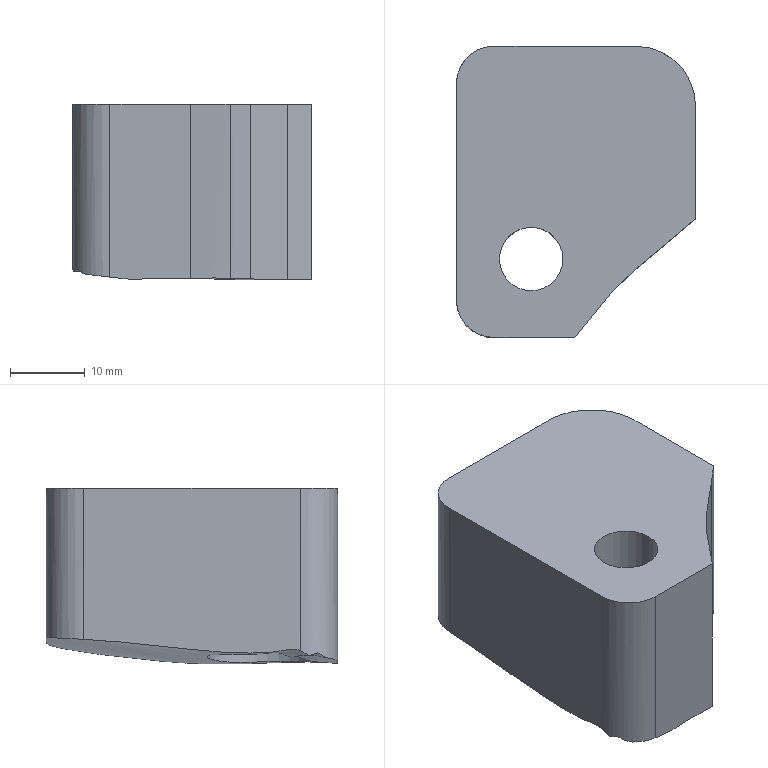Part | STEP file | gslz 2016.10.28-10_id2142_x_t | 1 solid | 16 faces | box 32 x 39 x 23.794 mm | volume 21462 mm3 | plane 6 | cylinder 5 | spline 4 | other 1 | commonest cylinder face diameters 10 x2 8.5 x1 14 x1 16 x1